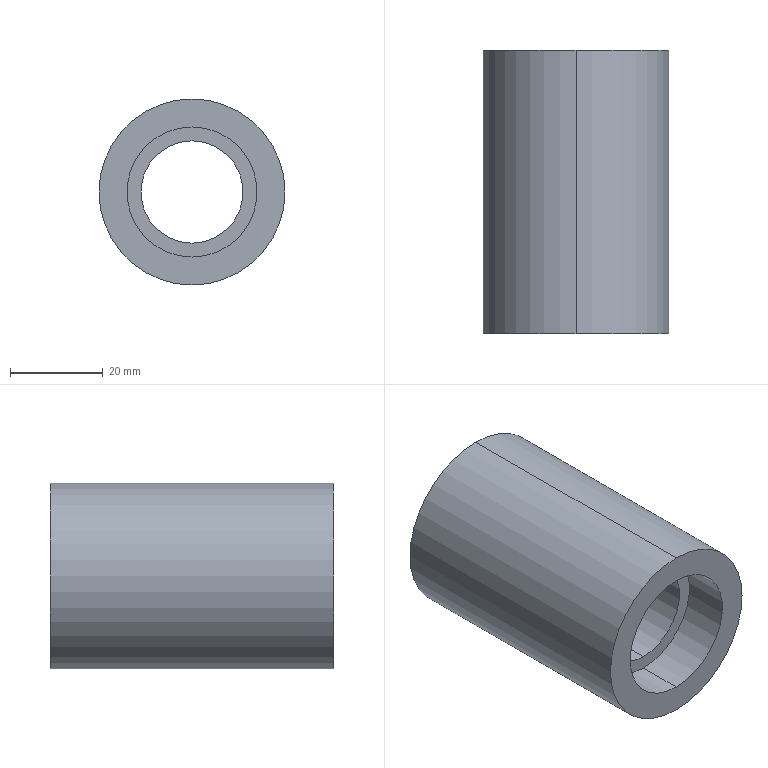Part | STEP file | ND25021-01-JDKM-22-TL | 1 solid | 12 faces | box 40 x 61 x 40 mm | volume 48754 mm3 | cylinder 8 | plane 4 | commonest cylinder face diameters 28 x4 22 x2 40 x2
STEP:
#1=CARTESIAN_POINT('',(0.,0.,0.));
#2=DIRECTION('',(0.,0.,1.));
#3=DIRECTION('',(1.,0.,0.));
#4=AXIS2_PLACEMENT_3D('',#1,#2,#3);
#5=CARTESIAN_POINT('',(0.,-20.5,-14.));
#6=VERTEX_POINT('',#5);
#7=CARTESIAN_POINT('',(0.,-30.5,-14.));
#8=VERTEX_POINT('',#7);
#9=CARTESIAN_POINT('',(0.,-20.5,-14.));
#10=DIRECTION('',(0.,-1.,0.));
#11=VECTOR('',#10,1.);
#12=LINE('',#9,#11);
#13=CARTESIAN_POINT('',(0.,-20.5,0.));
#14=DIRECTION('',(0.,-1.,0.));
#15=DIRECTION('',(0.,0.,-1.));
#16=AXIS2_PLACEMENT_3D('',#13,#14,#15);
#17=CYLINDRICAL_SURFACE('',#16,14.);
#18=CARTESIAN_POINT('',(6.283,0.));
#19=DIRECTION('',(0.,1.));
#20=VECTOR('',#19,1.);
#21=LINE('',#18,#20);
#22=(GEOMETRIC_REPRESENTATION_CONTEXT(2)PARAMETRIC_REPRESENTATION_CONTEXT()REPRESENTATION_CONTEXT('',''));
#23=DEFINITIONAL_REPRESENTATION('',(#21),#22);
#24=PCURVE('',#17,#23);
#25=CARTESIAN_POINT('',(0.,-20.5,0.));
#26=DIRECTION('',(0.,-1.,0.));
#27=DIRECTION('',(0.,0.,-1.));
#28=AXIS2_PLACEMENT_3D('',#25,#26,#27);
#29=CYLINDRICAL_SURFACE('',#28,14.);
#30=CARTESIAN_POINT('',(0.,0.));
#31=DIRECTION('',(0.,1.));
#32=VECTOR('',#31,1.);
#33=LINE('',#30,#32);
#34=(GEOMETRIC_REPRESENTATION_CONTEXT(2)PARAMETRIC_REPRESENTATION_CONTEXT()REPRESENTATION_CONTEXT('',''));
#35=DEFINITIONAL_REPRESENTATION('',(#33),#34);
#36=PCURVE('',#29,#35);
#37=SURFACE_CURVE('',#12,(#24,#36),.PCURVE_S1.);
#38=EDGE_CURVE('',#6,#8,#37,.T.);
#39=ORIENTED_EDGE('',*,*,#38,.T.);
#40=CARTESIAN_POINT('',(0.,-30.5,14.));
#41=VERTEX_POINT('',#40);
#42=CARTESIAN_POINT('',(0.,-30.5,0.));
#43=DIRECTION('',(0.,-1.,0.));
#44=DIRECTION('',(0.,0.,-1.));
#45=AXIS2_PLACEMENT_3D('',#42,#43,#44);
#46=CIRCLE('',#45,14.);
#47=CARTESIAN_POINT('',(0.,10.));
#48=DIRECTION('',(1.,0.));
#49=VECTOR('',#48,1.);
#50=LINE('',#47,#49);
#51=(GEOMETRIC_REPRESENTATION_CONTEXT(2)PARAMETRIC_REPRESENTATION_CONTEXT()REPRESENTATION_CONTEXT('',''));
#52=DEFINITIONAL_REPRESENTATION('',(#50),#51);
#53=PCURVE('',#17,#52);
#54=CARTESIAN_POINT('',(0.,-30.5,0.));
#55=DIRECTION('',(0.,1.,0.));
#56=DIRECTION('',(0.,0.,1.));
#57=AXIS2_PLACEMENT_3D('',#54,#55,#56);
#58=PLANE('',#57);
#59=CARTESIAN_POINT('',(-14.,0.));
#60=CARTESIAN_POINT('',(-14.,24.249));
#61=CARTESIAN_POINT('',(7.,12.124));
#62=CARTESIAN_POINT('',(28.,0.));
#63=CARTESIAN_POINT('',(7.,-12.124));
#64=CARTESIAN_POINT('',(-14.,-24.249));
#65=CARTESIAN_POINT('',(-14.,0.));
#66=(BOUNDED_CURVE()B_SPLINE_CURVE(2,(#59,#60,#61,#62,#63,#64,#65),.UNSPECIFIED.,.T.,.F.)B_SPLINE_CURVE_WITH_KNOTS((1,2,2,2,2,1),(-2.094,0.,2.094,4.189,6.283,8.378),.UNSPECIFIED.)CURVE()GEOMETRIC_REPRESENTATION_ITEM()RATIONAL_B_SPLINE_CURVE((1.,0.5,1.,0.5,1.,0.5,1.))REPRESENTATION_ITEM(''));
#67=(GEOMETRIC_REPRESENTATION_CONTEXT(2)PARAMETRIC_REPRESENTATION_CONTEXT()REPRESENTATION_CONTEXT('',''));
#68=DEFINITIONAL_REPRESENTATION('',(#66),#67);
#69=PCURVE('',#58,#68);
#70=SURFACE_CURVE('',#46,(#53,#69),.PCURVE_S1.);
#71=EDGE_CURVE('',#41,#8,#70,.T.);
#72=ORIENTED_EDGE('',*,*,#71,.F.);
#73=CARTESIAN_POINT('',(0.,-20.5,14.));
#74=VERTEX_POINT('',#73);
#75=CARTESIAN_POINT('',(0.,-20.5,14.));
#76=DIRECTION('',(0.,-1.,0.));
#77=VECTOR('',#76,1.);
#78=LINE('',#75,#77);
#79=CARTESIAN_POINT('',(3.142,0.));
#80=DIRECTION('',(0.,1.));
#81=VECTOR('',#80,1.);
#82=LINE('',#79,#81);
#83=(GEOMETRIC_REPRESENTATION_CONTEXT(2)PARAMETRIC_REPRESENTATION_CONTEXT()REPRESENTATION_CONTEXT('',''));
#84=DEFINITIONAL_REPRESENTATION('',(#82),#83);
#85=PCURVE('',#17,#84);
#86=CARTESIAN_POINT('',(3.142,0.));
#87=DIRECTION('',(0.,1.));
#88=VECTOR('',#87,1.);
#89=LINE('',#86,#88);
#90=(GEOMETRIC_REPRESENTATION_CONTEXT(2)PARAMETRIC_REPRESENTATION_CONTEXT()REPRESENTATION_CONTEXT('',''));
#91=DEFINITIONAL_REPRESENTATION('',(#89),#90);
#92=PCURVE('',#29,#91);
#93=SURFACE_CURVE('',#78,(#85,#92),.PCURVE_S1.);
#94=EDGE_CURVE('',#74,#41,#93,.T.);
#95=ORIENTED_EDGE('',*,*,#94,.F.);
#96=CARTESIAN_POINT('',(0.,-20.5,0.));
#97=DIRECTION('',(0.,-1.,0.));
#98=DIRECTION('',(0.,0.,-1.));
#99=AXIS2_PLACEMENT_3D('',#96,#97,#98);
#100=CIRCLE('',#99,14.);
#101=CARTESIAN_POINT('',(0.,0.));
#102=DIRECTION('',(1.,0.));
#103=VECTOR('',#102,1.);
#104=LINE('',#101,#103);
#105=(GEOMETRIC_REPRESENTATION_CONTEXT(2)PARAMETRIC_REPRESENTATION_CONTEXT()REPRESENTATION_CONTEXT('',''));
#106=DEFINITIONAL_REPRESENTATION('',(#104),#105);
#107=PCURVE('',#17,#106);
#108=CARTESIAN_POINT('',(0.,-20.5,0.));
#109=DIRECTION('',(0.,-1.,0.));
#110=DIRECTION('',(0.,0.,-1.));
#111=AXIS2_PLACEMENT_3D('',#108,#109,#110);
#112=PLANE('',#111);
#113=CARTESIAN_POINT('',(0.,0.));
#114=DIRECTION('',(1.,0.));
#115=AXIS2_PLACEMENT_2D('',#113,#114);
#116=CIRCLE('',#115,14.);
#117=(GEOMETRIC_REPRESENTATION_CONTEXT(2)PARAMETRIC_REPRESENTATION_CONTEXT()REPRESENTATION_CONTEXT('',''));
#118=DEFINITIONAL_REPRESENTATION('',(#116),#117);
#119=PCURVE('',#112,#118);
#120=SURFACE_CURVE('',#100,(#107,#119),.PCURVE_S1.);
#121=EDGE_CURVE('',#74,#6,#120,.T.);
#122=ORIENTED_EDGE('',*,*,#121,.T.);
#123=EDGE_LOOP('',(#39,#72,#95,#122));
#124=FACE_BOUND('',#123,.F.);
#125=ADVANCED_FACE('',(#124),#17,.F.);
#126=CARTESIAN_POINT('',(0.,20.5,14.));
#127=VERTEX_POINT('',#126);
#128=CARTESIAN_POINT('',(0.,30.5,14.));
#129=VERTEX_POINT('',#128);
#130=CARTESIAN_POINT('',(0.,20.5,14.));
#131=DIRECTION('',(0.,1.,0.));
#132=VECTOR('',#131,1.);
#133=LINE('',#130,#132);
#134=CARTESIAN_POINT('',(0.,20.5,0.));
#135=DIRECTION('',(0.,1.,0.));
#136=DIRECTION('',(0.,0.,1.));
#137=AXIS2_PLACEMENT_3D('',#134,#135,#136);
#138=CYLINDRICAL_SURFACE('',#137,14.);
#139=CARTESIAN_POINT('',(6.283,0.));
#140=DIRECTION('',(0.,1.));
#141=VECTOR('',#140,1.);
#142=LINE('',#139,#141);
#143=(GEOMETRIC_REPRESENTATION_CONTEXT(2)PARAMETRIC_REPRESENTATION_CONTEXT()REPRESENTATION_CONTEXT('',''));
#144=DEFINITIONAL_REPRESENTATION('',(#142),#143);
#145=PCURVE('',#138,#144);
#146=CARTESIAN_POINT('',(0.,20.5,0.));
#147=DIRECTION('',(0.,1.,0.));
#148=DIRECTION('',(0.,0.,1.));
#149=AXIS2_PLACEMENT_3D('',#146,#147,#148);
#150=CYLINDRICAL_SURFACE('',#149,14.);
#151=CARTESIAN_POINT('',(0.,0.));
#152=DIRECTION('',(0.,1.));
#153=VECTOR('',#152,1.);
#154=LINE('',#151,#153);
#155=(GEOMETRIC_REPRESENTATION_CONTEXT(2)PARAMETRIC_REPRESENTATION_CONTEXT()REPRESENTATION_CONTEXT('',''));
#156=DEFINITIONAL_REPRESENTATION('',(#154),#155);
#157=PCURVE('',#150,#156);
#158=SURFACE_CURVE('',#133,(#145,#157),.PCURVE_S1.);
#159=EDGE_CURVE('',#127,#129,#158,.T.);
#160=ORIENTED_EDGE('',*,*,#159,.T.);
#161=CARTESIAN_POINT('',(0.,30.5,-14.));
#162=VERTEX_POINT('',#161);
#163=CARTESIAN_POINT('',(0.,30.5,0.));
#164=DIRECTION('',(0.,1.,0.));
#165=DIRECTION('',(0.,0.,1.));
#166=AXIS2_PLACEMENT_3D('',#163,#164,#165);
#167=CIRCLE('',#166,14.);
#168=CARTESIAN_POINT('',(0.,10.));
#169=DIRECTION('',(1.,0.));
#170=VECTOR('',#169,1.);
#171=LINE('',#168,#170);
#172=(GEOMETRIC_REPRESENTATION_CONTEXT(2)PARAMETRIC_REPRESENTATION_CONTEXT()REPRESENTATION_CONTEXT('',''));
#173=DEFINITIONAL_REPRESENTATION('',(#171),#172);
#174=PCURVE('',#138,#173);
#175=CARTESIAN_POINT('',(0.,30.5,0.));
#176=DIRECTION('',(0.,1.,0.));
#177=DIRECTION('',(0.,0.,1.));
#178=AXIS2_PLACEMENT_3D('',#175,#176,#177);
#179=PLANE('',#178);
#180=CARTESIAN_POINT('',(0.,0.));
#181=DIRECTION('',(1.,0.));
#182=AXIS2_PLACEMENT_2D('',#180,#181);
#183=CIRCLE('',#182,14.);
#184=(GEOMETRIC_REPRESENTATION_CONTEXT(2)PARAMETRIC_REPRESENTATION_CONTEXT()REPRESENTATION_CONTEXT('',''));
#185=DEFINITIONAL_REPRESENTATION('',(#183),#184);
#186=PCURVE('',#179,#185);
#187=SURFACE_CURVE('',#167,(#174,#186),.PCURVE_S1.);
#188=EDGE_CURVE('',#162,#129,#187,.T.);
#189=ORIENTED_EDGE('',*,*,#188,.F.);
#190=CARTESIAN_POINT('',(0.,20.5,-14.));
#191=VERTEX_POINT('',#190);
#192=CARTESIAN_POINT('',(0.,20.5,-14.));
#193=DIRECTION('',(0.,1.,0.));
#194=VECTOR('',#193,1.);
#195=LINE('',#192,#194);
#196=CARTESIAN_POINT('',(3.142,0.));
#197=DIRECTION('',(0.,1.));
#198=VECTOR('',#197,1.);
#199=LINE('',#196,#198);
#200=(GEOMETRIC_REPRESENTATION_CONTEXT(2)PARAMETRIC_REPRESENTATION_CONTEXT()REPRESENTATION_CONTEXT('',''));
#201=DEFINITIONAL_REPRESENTATION('',(#199),#200);
#202=PCURVE('',#138,#201);
#203=CARTESIAN_POINT('',(3.142,0.));
#204=DIRECTION('',(0.,1.));
#205=VECTOR('',#204,1.);
#206=LINE('',#203,#205);
#207=(GEOMETRIC_REPRESENTATION_CONTEXT(2)PARAMETRIC_REPRESENTATION_CONTEXT()REPRESENTATION_CONTEXT('',''));
#208=DEFINITIONAL_REPRESENTATION('',(#206),#207);
#209=PCURVE('',#150,#208);
#210=SURFACE_CURVE('',#195,(#202,#209),.PCURVE_S1.);
#211=EDGE_CURVE('',#191,#162,#210,.T.);
#212=ORIENTED_EDGE('',*,*,#211,.F.);
#213=CARTESIAN_POINT('',(0.,20.5,0.));
#214=DIRECTION('',(0.,1.,0.));
#215=DIRECTION('',(0.,0.,1.));
#216=AXIS2_PLACEMENT_3D('',#213,#214,#215);
#217=CIRCLE('',#216,14.);
#218=CARTESIAN_POINT('',(0.,0.));
#219=DIRECTION('',(1.,0.));
#220=VECTOR('',#219,1.);
#221=LINE('',#218,#220);
#222=(GEOMETRIC_REPRESENTATION_CONTEXT(2)PARAMETRIC_REPRESENTATION_CONTEXT()REPRESENTATION_CONTEXT('',''));
#223=DEFINITIONAL_REPRESENTATION('',(#221),#222);
#224=PCURVE('',#138,#223);
#225=CARTESIAN_POINT('',(0.,20.5,0.));
#226=DIRECTION('',(0.,1.,0.));
#227=DIRECTION('',(0.,0.,1.));
#228=AXIS2_PLACEMENT_3D('',#225,#226,#227);
#229=PLANE('',#228);
#230=CARTESIAN_POINT('',(0.,0.));
#231=DIRECTION('',(1.,0.));
#232=AXIS2_PLACEMENT_2D('',#230,#231);
#233=CIRCLE('',#232,14.);
#234=(GEOMETRIC_REPRESENTATION_CONTEXT(2)PARAMETRIC_REPRESENTATION_CONTEXT()REPRESENTATION_CONTEXT('',''));
#235=DEFINITIONAL_REPRESENTATION('',(#233),#234);
#236=PCURVE('',#229,#235);
#237=SURFACE_CURVE('',#217,(#224,#236),.PCURVE_S1.);
#238=EDGE_CURVE('',#191,#127,#237,.T.);
#239=ORIENTED_EDGE('',*,*,#238,.T.);
#240=EDGE_LOOP('',(#160,#189,#212,#239));
#241=FACE_BOUND('',#240,.F.);
#242=ADVANCED_FACE('',(#241),#138,.F.);
#243=CARTESIAN_POINT('',(0.,30.5,20.));
#244=VERTEX_POINT('',#243);
#245=CARTESIAN_POINT('',(0.,30.5,-20.));
#246=VERTEX_POINT('',#245);
#247=CARTESIAN_POINT('',(0.,30.5,0.));
#248=DIRECTION('',(0.,1.,0.));
#249=DIRECTION('',(0.,0.,1.));
#250=AXIS2_PLACEMENT_3D('',#247,#248,#249);
#251=CIRCLE('',#250,20.);
#252=CARTESIAN_POINT('',(0.,30.5,0.));
#253=DIRECTION('',(0.,-1.,0.));
#254=DIRECTION('',(0.,0.,-1.));
#255=AXIS2_PLACEMENT_3D('',#252,#253,#254);
#256=CYLINDRICAL_SURFACE('',#255,20.);
#257=CARTESIAN_POINT('',(3.142,0.));
#258=DIRECTION('',(-1.,0.));
#259=VECTOR('',#258,1.);
#260=LINE('',#257,#259);
#261=(GEOMETRIC_REPRESENTATION_CONTEXT(2)PARAMETRIC_REPRESENTATION_CONTEXT()REPRESENTATION_CONTEXT('',''));
#262=DEFINITIONAL_REPRESENTATION('',(#260),#261);
#263=PCURVE('',#256,#262);
#264=CARTESIAN_POINT('',(0.,0.));
#265=DIRECTION('',(1.,0.));
#266=AXIS2_PLACEMENT_2D('',#264,#265);
#267=CIRCLE('',#266,20.);
#268=(GEOMETRIC_REPRESENTATION_CONTEXT(2)PARAMETRIC_REPRESENTATION_CONTEXT()REPRESENTATION_CONTEXT('',''));
#269=DEFINITIONAL_REPRESENTATION('',(#267),#268);
#270=PCURVE('',#179,#269);
#271=SURFACE_CURVE('',#251,(#263,#270),.PCURVE_S1.);
#272=EDGE_CURVE('',#244,#246,#271,.T.);
#273=ORIENTED_EDGE('',*,*,#272,.F.);
#274=CARTESIAN_POINT('',(0.,-30.5,20.));
#275=VERTEX_POINT('',#274);
#276=CARTESIAN_POINT('',(0.,30.5,20.));
#277=DIRECTION('',(0.,-1.,0.));
#278=VECTOR('',#277,1.);
#279=LINE('',#276,#278);
#280=CARTESIAN_POINT('',(3.142,0.));
#281=DIRECTION('',(0.,1.));
#282=VECTOR('',#281,1.);
#283=LINE('',#280,#282);
#284=(GEOMETRIC_REPRESENTATION_CONTEXT(2)PARAMETRIC_REPRESENTATION_CONTEXT()REPRESENTATION_CONTEXT('',''));
#285=DEFINITIONAL_REPRESENTATION('',(#283),#284);
#286=PCURVE('',#256,#285);
#287=CARTESIAN_POINT('',(0.,30.5,0.));
#288=DIRECTION('',(0.,-1.,0.));
#289=DIRECTION('',(0.,0.,-1.));
#290=AXIS2_PLACEMENT_3D('',#287,#288,#289);
#291=CYLINDRICAL_SURFACE('',#290,20.);
#292=CARTESIAN_POINT('',(3.142,0.));
#293=DIRECTION('',(0.,1.));
#294=VECTOR('',#293,1.);
#295=LINE('',#292,#294);
#296=(GEOMETRIC_REPRESENTATION_CONTEXT(2)PARAMETRIC_REPRESENTATION_CONTEXT()REPRESENTATION_CONTEXT('',''));
#297=DEFINITIONAL_REPRESENTATION('',(#295),#296);
#298=PCURVE('',#291,#297);
#299=SURFACE_CURVE('',#279,(#286,#298),.PCURVE_S1.);
#300=EDGE_CURVE('',#244,#275,#299,.T.);
#301=ORIENTED_EDGE('',*,*,#300,.T.);
#302=CARTESIAN_POINT('',(0.,-30.5,-20.));
#303=VERTEX_POINT('',#302);
#304=CARTESIAN_POINT('',(0.,-30.5,0.));
#305=DIRECTION('',(0.,1.,0.));
#306=DIRECTION('',(0.,0.,1.));
#307=AXIS2_PLACEMENT_3D('',#304,#305,#306);
#308=CIRCLE('',#307,20.);
#309=CARTESIAN_POINT('',(3.142,61.));
#310=DIRECTION('',(-1.,0.));
#311=VECTOR('',#310,1.);
#312=LINE('',#309,#311);
#313=(GEOMETRIC_REPRESENTATION_CONTEXT(2)PARAMETRIC_REPRESENTATION_CONTEXT()REPRESENTATION_CONTEXT('',''));
#314=DEFINITIONAL_REPRESENTATION('',(#312),#313);
#315=PCURVE('',#256,#314);
#316=CARTESIAN_POINT('',(0.,0.));
#317=DIRECTION('',(1.,0.));
#318=AXIS2_PLACEMENT_2D('',#316,#317);
#319=CIRCLE('',#318,20.);
#320=(GEOMETRIC_REPRESENTATION_CONTEXT(2)PARAMETRIC_REPRESENTATION_CONTEXT()REPRESENTATION_CONTEXT('',''));
#321=DEFINITIONAL_REPRESENTATION('',(#319),#320);
#322=PCURVE('',#58,#321);
#323=SURFACE_CURVE('',#308,(#315,#322),.PCURVE_S1.);
#324=EDGE_CURVE('',#275,#303,#323,.T.);
#325=ORIENTED_EDGE('',*,*,#324,.T.);
#326=CARTESIAN_POINT('',(0.,30.5,-20.));
#327=DIRECTION('',(0.,-1.,0.));
#328=VECTOR('',#327,1.);
#329=LINE('',#326,#328);
#330=CARTESIAN_POINT('',(0.,0.));
#331=DIRECTION('',(0.,1.));
#332=VECTOR('',#331,1.);
#333=LINE('',#330,#332);
#334=(GEOMETRIC_REPRESENTATION_CONTEXT(2)PARAMETRIC_REPRESENTATION_CONTEXT()REPRESENTATION_CONTEXT('',''));
#335=DEFINITIONAL_REPRESENTATION('',(#333),#334);
#336=PCURVE('',#256,#335);
#337=CARTESIAN_POINT('',(6.283,0.));
#338=DIRECTION('',(0.,1.));
#339=VECTOR('',#338,1.);
#340=LINE('',#337,#339);
#341=(GEOMETRIC_REPRESENTATION_CONTEXT(2)PARAMETRIC_REPRESENTATION_CONTEXT()REPRESENTATION_CONTEXT('',''));
#342=DEFINITIONAL_REPRESENTATION('',(#340),#341);
#343=PCURVE('',#291,#342);
#344=SURFACE_CURVE('',#329,(#336,#343),.PCURVE_S1.);
#345=EDGE_CURVE('',#246,#303,#344,.T.);
#346=ORIENTED_EDGE('',*,*,#345,.F.);
#347=EDGE_LOOP('',(#273,#301,#325,#346));
#348=FACE_BOUND('',#347,.T.);
#349=ADVANCED_FACE('',(#348),#256,.T.);
#350=CARTESIAN_POINT('',(0.,-20.5,11.));
#351=VERTEX_POINT('',#350);
#352=CARTESIAN_POINT('',(0.,20.5,11.));
#353=VERTEX_POINT('',#352);
#354=CARTESIAN_POINT('',(0.,-30.5,11.));
#355=DIRECTION('',(0.,1.,0.));
#356=VECTOR('',#355,1.);
#357=LINE('',#354,#356);
#358=CARTESIAN_POINT('',(0.,-30.5,0.));
#359=DIRECTION('',(0.,1.,0.));
#360=DIRECTION('',(0.,0.,1.));
#361=AXIS2_PLACEMENT_3D('',#358,#359,#360);
#362=CYLINDRICAL_SURFACE('',#361,11.);
#363=CARTESIAN_POINT('',(6.283,0.));
#364=DIRECTION('',(0.,1.));
#365=VECTOR('',#364,1.);
#366=LINE('',#363,#365);
#367=(GEOMETRIC_REPRESENTATION_CONTEXT(2)PARAMETRIC_REPRESENTATION_CONTEXT()REPRESENTATION_CONTEXT('',''));
#368=DEFINITIONAL_REPRESENTATION('',(#366),#367);
#369=PCURVE('',#362,#368);
#370=CARTESIAN_POINT('',(0.,-30.5,0.));
#371=DIRECTION('',(0.,1.,0.));
#372=DIRECTION('',(0.,0.,1.));
#373=AXIS2_PLACEMENT_3D('',#370,#371,#372);
#374=CYLINDRICAL_SURFACE('',#373,11.);
#375=CARTESIAN_POINT('',(0.,0.));
#376=DIRECTION('',(0.,1.));
#377=VECTOR('',#376,1.);
#378=LINE('',#375,#377);
#379=(GEOMETRIC_REPRESENTATION_CONTEXT(2)PARAMETRIC_REPRESENTATION_CONTEXT()REPRESENTATION_CONTEXT('',''));
#380=DEFINITIONAL_REPRESENTATION('',(#378),#379);
#381=PCURVE('',#374,#380);
#382=SURFACE_CURVE('',#357,(#369,#381),.PCURVE_S1.);
#383=EDGE_CURVE('',#351,#353,#382,.T.);
#384=ORIENTED_EDGE('',*,*,#383,.T.);
#385=CARTESIAN_POINT('',(0.,20.5,-11.));
#386=VERTEX_POINT('',#385);
#387=CARTESIAN_POINT('',(0.,20.5,0.));
#388=DIRECTION('',(0.,-1.,0.));
#389=DIRECTION('',(0.,0.,1.));
#390=AXIS2_PLACEMENT_3D('',#387,#388,#389);
#391=CIRCLE('',#390,11.);
#392=CARTESIAN_POINT('',(6.283,51.));
#393=DIRECTION('',(-1.,0.));
#394=VECTOR('',#393,1.);
#395=LINE('',#392,#394);
#396=(GEOMETRIC_REPRESENTATION_CONTEXT(2)PARAMETRIC_REPRESENTATION_CONTEXT()REPRESENTATION_CONTEXT('',''));
#397=DEFINITIONAL_REPRESENTATION('',(#395),#396);
#398=PCURVE('',#362,#397);
#399=CARTESIAN_POINT('',(11.,0.));
#400=CARTESIAN_POINT('',(11.,-19.053));
#401=CARTESIAN_POINT('',(-5.5,-9.526));
#402=CARTESIAN_POINT('',(-22.,0.));
#403=CARTESIAN_POINT('',(-5.5,9.526));
#404=CARTESIAN_POINT('',(11.,19.053));
#405=CARTESIAN_POINT('',(11.,0.));
#406=(BOUNDED_CURVE()B_SPLINE_CURVE(2,(#399,#400,#401,#402,#403,#404,#405),.UNSPECIFIED.,.T.,.F.)B_SPLINE_CURVE_WITH_KNOTS((1,2,2,2,2,1),(-2.094,0.,2.094,4.189,6.283,8.378),.UNSPECIFIED.)CURVE()GEOMETRIC_REPRESENTATION_ITEM()RATIONAL_B_SPLINE_CURVE((1.,0.5,1.,0.5,1.,0.5,1.))REPRESENTATION_ITEM(''));
#407=(GEOMETRIC_REPRESENTATION_CONTEXT(2)PARAMETRIC_REPRESENTATION_CONTEXT()REPRESENTATION_CONTEXT('',''));
#408=DEFINITIONAL_REPRESENTATION('',(#406),#407);
#409=PCURVE('',#229,#408);
#410=SURFACE_CURVE('',#391,(#398,#409),.PCURVE_S1.);
#411=EDGE_CURVE('',#353,#386,#410,.T.);
#412=ORIENTED_EDGE('',*,*,#411,.T.);
#413=CARTESIAN_POINT('',(0.,-20.5,-11.));
#414=VERTEX_POINT('',#413);
#415=CARTESIAN_POINT('',(0.,-30.5,-11.));
#416=DIRECTION('',(0.,1.,0.));
#417=VECTOR('',#416,1.);
#418=LINE('',#415,#417);
#419=CARTESIAN_POINT('',(3.142,0.));
#420=DIRECTION('',(0.,1.));
#421=VECTOR('',#420,1.);
#422=LINE('',#419,#421);
#423=(GEOMETRIC_REPRESENTATION_CONTEXT(2)PARAMETRIC_REPRESENTATION_CONTEXT()REPRESENTATION_CONTEXT('',''));
#424=DEFINITIONAL_REPRESENTATION('',(#422),#423);
#425=PCURVE('',#362,#424);
#426=CARTESIAN_POINT('',(3.142,0.));
#427=DIRECTION('',(0.,1.));
#428=VECTOR('',#427,1.);
#429=LINE('',#426,#428);
#430=(GEOMETRIC_REPRESENTATION_CONTEXT(2)PARAMETRIC_REPRESENTATION_CONTEXT()REPRESENTATION_CONTEXT('',''));
#431=DEFINITIONAL_REPRESENTATION('',(#429),#430);
#432=PCURVE('',#374,#431);
#433=SURFACE_CURVE('',#418,(#425,#432),.PCURVE_S1.);
#434=EDGE_CURVE('',#414,#386,#433,.T.);
#435=ORIENTED_EDGE('',*,*,#434,.F.);
#436=CARTESIAN_POINT('',(0.,-20.5,0.));
#437=DIRECTION('',(0.,1.,0.));
#438=DIRECTION('',(0.,0.,-1.));
#439=AXIS2_PLACEMENT_3D('',#436,#437,#438);
#440=CIRCLE('',#439,11.);
#441=CARTESIAN_POINT('',(3.142,10.));
#442=DIRECTION('',(1.,0.));
#443=VECTOR('',#442,1.);
#444=LINE('',#441,#443);
#445=(GEOMETRIC_REPRESENTATION_CONTEXT(2)PARAMETRIC_REPRESENTATION_CONTEXT()REPRESENTATION_CONTEXT('',''));
#446=DEFINITIONAL_REPRESENTATION('',(#444),#445);
#447=PCURVE('',#362,#446);
#448=CARTESIAN_POINT('',(11.,0.));
#449=CARTESIAN_POINT('',(11.,-19.053));
#450=CARTESIAN_POINT('',(-5.5,-9.526));
#451=CARTESIAN_POINT('',(-22.,0.));
#452=CARTESIAN_POINT('',(-5.5,9.526));
#453=CARTESIAN_POINT('',(11.,19.053));
#454=CARTESIAN_POINT('',(11.,0.));
#455=(BOUNDED_CURVE()B_SPLINE_CURVE(2,(#448,#449,#450,#451,#452,#453,#454),.UNSPECIFIED.,.T.,.F.)B_SPLINE_CURVE_WITH_KNOTS((1,2,2,2,2,1),(-2.094,0.,2.094,4.189,6.283,8.378),.UNSPECIFIED.)CURVE()GEOMETRIC_REPRESENTATION_ITEM()RATIONAL_B_SPLINE_CURVE((1.,0.5,1.,0.5,1.,0.5,1.))REPRESENTATION_ITEM(''));
#456=(GEOMETRIC_REPRESENTATION_CONTEXT(2)PARAMETRIC_REPRESENTATION_CONTEXT()REPRESENTATION_CONTEXT('',''));
#457=DEFINITIONAL_REPRESENTATION('',(#455),#456);
#458=PCURVE('',#112,#457);
#459=SURFACE_CURVE('',#440,(#447,#458),.PCURVE_S1.);
#460=EDGE_CURVE('',#414,#351,#459,.T.);
#461=ORIENTED_EDGE('',*,*,#460,.T.);
#462=EDGE_LOOP('',(#384,#412,#435,#461));
#463=FACE_BOUND('',#462,.F.);
#464=ADVANCED_FACE('',(#463),#362,.F.);
#465=CARTESIAN_POINT('',(0.,20.5,0.));
#466=DIRECTION('',(0.,-1.,0.));
#467=DIRECTION('',(0.,0.,1.));
#468=AXIS2_PLACEMENT_3D('',#465,#466,#467);
#469=CIRCLE('',#468,11.);
#470=CARTESIAN_POINT('',(6.283,51.));
#471=DIRECTION('',(-1.,0.));
#472=VECTOR('',#471,1.);
#473=LINE('',#470,#472);
#474=(GEOMETRIC_REPRESENTATION_CONTEXT(2)PARAMETRIC_REPRESENTATION_CONTEXT()REPRESENTATION_CONTEXT('',''));
#475=DEFINITIONAL_REPRESENTATION('',(#473),#474);
#476=PCURVE('',#374,#475);
#477=CARTESIAN_POINT('',(11.,0.));
#478=CARTESIAN_POINT('',(11.,-19.053));
#479=CARTESIAN_POINT('',(-5.5,-9.526));
#480=CARTESIAN_POINT('',(-22.,0.));
#481=CARTESIAN_POINT('',(-5.5,9.526));
#482=CARTESIAN_POINT('',(11.,19.053));
#483=CARTESIAN_POINT('',(11.,0.));
#484=(BOUNDED_CURVE()B_SPLINE_CURVE(2,(#477,#478,#479,#480,#481,#482,#483),.UNSPECIFIED.,.T.,.F.)B_SPLINE_CURVE_WITH_KNOTS((1,2,2,2,2,1),(-2.094,0.,2.094,4.189,6.283,8.378),.UNSPECIFIED.)CURVE()GEOMETRIC_REPRESENTATION_ITEM()RATIONAL_B_SPLINE_CURVE((1.,0.5,1.,0.5,1.,0.5,1.))REPRESENTATION_ITEM(''));
#485=(GEOMETRIC_REPRESENTATION_CONTEXT(2)PARAMETRIC_REPRESENTATION_CONTEXT()REPRESENTATION_CONTEXT('',''));
#486=DEFINITIONAL_REPRESENTATION('',(#484),#485);
#487=PCURVE('',#229,#486);
#488=SURFACE_CURVE('',#469,(#476,#487),.PCURVE_S1.);
#489=EDGE_CURVE('',#386,#353,#488,.T.);
#490=ORIENTED_EDGE('',*,*,#489,.T.);
#491=ORIENTED_EDGE('',*,*,#383,.F.);
#492=CARTESIAN_POINT('',(0.,-20.5,0.));
#493=DIRECTION('',(0.,1.,0.));
#494=DIRECTION('',(0.,0.,-1.));
#495=AXIS2_PLACEMENT_3D('',#492,#493,#494);
#496=CIRCLE('',#495,11.);
#497=CARTESIAN_POINT('',(-3.142,10.));
#498=DIRECTION('',(1.,0.));
#499=VECTOR('',#498,1.);
#500=LINE('',#497,#499);
#501=(GEOMETRIC_REPRESENTATION_CONTEXT(2)PARAMETRIC_REPRESENTATION_CONTEXT()REPRESENTATION_CONTEXT('',''));
#502=DEFINITIONAL_REPRESENTATION('',(#500),#501);
#503=PCURVE('',#374,#502);
#504=CARTESIAN_POINT('',(11.,0.));
#505=CARTESIAN_POINT('',(11.,-19.053));
#506=CARTESIAN_POINT('',(-5.5,-9.526));
#507=CARTESIAN_POINT('',(-22.,0.));
#508=CARTESIAN_POINT('',(-5.5,9.526));
#509=CARTESIAN_POINT('',(11.,19.053));
#510=CARTESIAN_POINT('',(11.,0.));
#511=(BOUNDED_CURVE()B_SPLINE_CURVE(2,(#504,#505,#506,#507,#508,#509,#510),.UNSPECIFIED.,.T.,.F.)B_SPLINE_CURVE_WITH_KNOTS((1,2,2,2,2,1),(-2.094,0.,2.094,4.189,6.283,8.378),.UNSPECIFIED.)CURVE()GEOMETRIC_REPRESENTATION_ITEM()RATIONAL_B_SPLINE_CURVE((1.,0.5,1.,0.5,1.,0.5,1.))REPRESENTATION_ITEM(''));
#512=(GEOMETRIC_REPRESENTATION_CONTEXT(2)PARAMETRIC_REPRESENTATION_CONTEXT()REPRESENTATION_CONTEXT('',''));
#513=DEFINITIONAL_REPRESENTATION('',(#511),#512);
#514=PCURVE('',#112,#513);
#515=SURFACE_CURVE('',#496,(#503,#514),.PCURVE_S1.);
#516=EDGE_CURVE('',#351,#414,#515,.T.);
#517=ORIENTED_EDGE('',*,*,#516,.T.);
#518=ORIENTED_EDGE('',*,*,#434,.T.);
#519=EDGE_LOOP('',(#490,#491,#517,#518));
#520=FACE_BOUND('',#519,.F.);
#521=ADVANCED_FACE('',(#520),#374,.F.);
#522=ORIENTED_EDGE('',*,*,#300,.F.);
#523=CARTESIAN_POINT('',(0.,30.5,0.));
#524=DIRECTION('',(0.,1.,0.));
#525=DIRECTION('',(0.,0.,1.));
#526=AXIS2_PLACEMENT_3D('',#523,#524,#525);
#527=CIRCLE('',#526,20.);
#528=CARTESIAN_POINT('',(9.425,0.));
#529=DIRECTION('',(-1.,0.));
#530=VECTOR('',#529,1.);
#531=LINE('',#528,#530);
#532=(GEOMETRIC_REPRESENTATION_CONTEXT(2)PARAMETRIC_REPRESENTATION_CONTEXT()REPRESENTATION_CONTEXT('',''));
#533=DEFINITIONAL_REPRESENTATION('',(#531),#532);
#534=PCURVE('',#291,#533);
#535=CARTESIAN_POINT('',(0.,0.));
#536=DIRECTION('',(1.,0.));
#537=AXIS2_PLACEMENT_2D('',#535,#536);
#538=CIRCLE('',#537,20.);
#539=(GEOMETRIC_REPRESENTATION_CONTEXT(2)PARAMETRIC_REPRESENTATION_CONTEXT()REPRESENTATION_CONTEXT('',''));
#540=DEFINITIONAL_REPRESENTATION('',(#538),#539);
#541=PCURVE('',#179,#540);
#542=SURFACE_CURVE('',#527,(#534,#541),.PCURVE_S1.);
#543=EDGE_CURVE('',#246,#244,#542,.T.);
#544=ORIENTED_EDGE('',*,*,#543,.F.);
#545=ORIENTED_EDGE('',*,*,#345,.T.);
#546=CARTESIAN_POINT('',(0.,-30.5,0.));
#547=DIRECTION('',(0.,1.,0.));
#548=DIRECTION('',(0.,0.,1.));
#549=AXIS2_PLACEMENT_3D('',#546,#547,#548);
#550=CIRCLE('',#549,20.);
#551=CARTESIAN_POINT('',(9.425,61.));
#552=DIRECTION('',(-1.,0.));
#553=VECTOR('',#552,1.);
#554=LINE('',#551,#553);
#555=(GEOMETRIC_REPRESENTATION_CONTEXT(2)PARAMETRIC_REPRESENTATION_CONTEXT()REPRESENTATION_CONTEXT('',''));
#556=DEFINITIONAL_REPRESENTATION('',(#554),#555);
#557=PCURVE('',#291,#556);
#558=CARTESIAN_POINT('',(0.,0.));
#559=DIRECTION('',(1.,0.));
#560=AXIS2_PLACEMENT_2D('',#558,#559);
#561=CIRCLE('',#560,20.);
#562=(GEOMETRIC_REPRESENTATION_CONTEXT(2)PARAMETRIC_REPRESENTATION_CONTEXT()REPRESENTATION_CONTEXT('',''));
#563=DEFINITIONAL_REPRESENTATION('',(#561),#562);
#564=PCURVE('',#58,#563);
#565=SURFACE_CURVE('',#550,(#557,#564),.PCURVE_S1.);
#566=EDGE_CURVE('',#303,#275,#565,.T.);
#567=ORIENTED_EDGE('',*,*,#566,.T.);
#568=EDGE_LOOP('',(#522,#544,#545,#567));
#569=FACE_BOUND('',#568,.T.);
#570=ADVANCED_FACE('',(#569),#291,.T.);
#571=CARTESIAN_POINT('',(0.,30.5,0.));
#572=DIRECTION('',(0.,1.,0.));
#573=DIRECTION('',(0.,0.,1.));
#574=AXIS2_PLACEMENT_3D('',#571,#572,#573);
#575=CIRCLE('',#574,14.);
#576=CARTESIAN_POINT('',(0.,0.));
#577=DIRECTION('',(1.,0.));
#578=AXIS2_PLACEMENT_2D('',#576,#577);
#579=CIRCLE('',#578,14.);
#580=(GEOMETRIC_REPRESENTATION_CONTEXT(2)PARAMETRIC_REPRESENTATION_CONTEXT()REPRESENTATION_CONTEXT('',''));
#581=DEFINITIONAL_REPRESENTATION('',(#579),#580);
#582=PCURVE('',#179,#581);
#583=CARTESIAN_POINT('',(0.,10.));
#584=DIRECTION('',(1.,0.));
#585=VECTOR('',#584,1.);
#586=LINE('',#583,#585);
#587=(GEOMETRIC_REPRESENTATION_CONTEXT(2)PARAMETRIC_REPRESENTATION_CONTEXT()REPRESENTATION_CONTEXT('',''));
#588=DEFINITIONAL_REPRESENTATION('',(#586),#587);
#589=PCURVE('',#150,#588);
#590=SURFACE_CURVE('',#575,(#582,#589),.PCURVE_S1.);
#591=EDGE_CURVE('',#129,#162,#590,.T.);
#592=ORIENTED_EDGE('',*,*,#591,.F.);
#593=ORIENTED_EDGE('',*,*,#188,.F.);
#594=EDGE_LOOP('',(#592,#593));
#595=FACE_BOUND('',#594,.T.);
#596=ORIENTED_EDGE('',*,*,#543,.T.);
#597=ORIENTED_EDGE('',*,*,#272,.T.);
#598=EDGE_LOOP('',(#596,#597));
#599=FACE_BOUND('',#598,.T.);
#600=ADVANCED_FACE('',(#595,#599),#179,.T.);
#601=CARTESIAN_POINT('',(0.,-30.5,0.));
#602=DIRECTION('',(0.,-1.,0.));
#603=DIRECTION('',(0.,0.,-1.));
#604=AXIS2_PLACEMENT_3D('',#601,#602,#603);
#605=CIRCLE('',#604,14.);
#606=CARTESIAN_POINT('',(-14.,0.));
#607=CARTESIAN_POINT('',(-14.,24.249));
#608=CARTESIAN_POINT('',(7.,12.124));
#609=CARTESIAN_POINT('',(28.,0.));
#610=CARTESIAN_POINT('',(7.,-12.124));
#611=CARTESIAN_POINT('',(-14.,-24.249));
#612=CARTESIAN_POINT('',(-14.,0.));
#613=(BOUNDED_CURVE()B_SPLINE_CURVE(2,(#606,#607,#608,#609,#610,#611,#612),.UNSPECIFIED.,.T.,.F.)B_SPLINE_CURVE_WITH_KNOTS((1,2,2,2,2,1),(-2.094,0.,2.094,4.189,6.283,8.378),.UNSPECIFIED.)CURVE()GEOMETRIC_REPRESENTATION_ITEM()RATIONAL_B_SPLINE_CURVE((1.,0.5,1.,0.5,1.,0.5,1.))REPRESENTATION_ITEM(''));
#614=(GEOMETRIC_REPRESENTATION_CONTEXT(2)PARAMETRIC_REPRESENTATION_CONTEXT()REPRESENTATION_CONTEXT('',''));
#615=DEFINITIONAL_REPRESENTATION('',(#613),#614);
#616=PCURVE('',#58,#615);
#617=CARTESIAN_POINT('',(0.,10.));
#618=DIRECTION('',(1.,0.));
#619=VECTOR('',#618,1.);
#620=LINE('',#617,#619);
#621=(GEOMETRIC_REPRESENTATION_CONTEXT(2)PARAMETRIC_REPRESENTATION_CONTEXT()REPRESENTATION_CONTEXT('',''));
#622=DEFINITIONAL_REPRESENTATION('',(#620),#621);
#623=PCURVE('',#29,#622);
#624=SURFACE_CURVE('',#605,(#616,#623),.PCURVE_S1.);
#625=EDGE_CURVE('',#8,#41,#624,.T.);
#626=ORIENTED_EDGE('',*,*,#625,.F.);
#627=ORIENTED_EDGE('',*,*,#71,.F.);
#628=EDGE_LOOP('',(#626,#627));
#629=FACE_BOUND('',#628,.T.);
#630=ORIENTED_EDGE('',*,*,#566,.F.);
#631=ORIENTED_EDGE('',*,*,#324,.F.);
#632=EDGE_LOOP('',(#630,#631));
#633=FACE_BOUND('',#632,.T.);
#634=ADVANCED_FACE('',(#629,#633),#58,.F.);
#635=CARTESIAN_POINT('',(0.,20.5,0.));
#636=DIRECTION('',(0.,1.,0.));
#637=DIRECTION('',(0.,0.,1.));
#638=AXIS2_PLACEMENT_3D('',#635,#636,#637);
#639=CIRCLE('',#638,14.);
#640=CARTESIAN_POINT('',(0.,0.));
#641=DIRECTION('',(1.,0.));
#642=AXIS2_PLACEMENT_2D('',#640,#641);
#643=CIRCLE('',#642,14.);
#644=(GEOMETRIC_REPRESENTATION_CONTEXT(2)PARAMETRIC_REPRESENTATION_CONTEXT()REPRESENTATION_CONTEXT('',''));
#645=DEFINITIONAL_REPRESENTATION('',(#643),#644);
#646=PCURVE('',#229,#645);
#647=CARTESIAN_POINT('',(0.,0.));
#648=DIRECTION('',(1.,0.));
#649=VECTOR('',#648,1.);
#650=LINE('',#647,#649);
#651=(GEOMETRIC_REPRESENTATION_CONTEXT(2)PARAMETRIC_REPRESENTATION_CONTEXT()REPRESENTATION_CONTEXT('',''));
#652=DEFINITIONAL_REPRESENTATION('',(#650),#651);
#653=PCURVE('',#150,#652);
#654=SURFACE_CURVE('',#639,(#646,#653),.PCURVE_S1.);
#655=EDGE_CURVE('',#127,#191,#654,.T.);
#656=ORIENTED_EDGE('',*,*,#655,.T.);
#657=ORIENTED_EDGE('',*,*,#238,.T.);
#658=EDGE_LOOP('',(#656,#657));
#659=FACE_BOUND('',#658,.T.);
#660=ORIENTED_EDGE('',*,*,#411,.T.);
#661=ORIENTED_EDGE('',*,*,#489,.T.);
#662=EDGE_LOOP('',(#660,#661));
#663=FACE_BOUND('',#662,.T.);
#664=ADVANCED_FACE('',(#659,#663),#229,.T.);
#665=ORIENTED_EDGE('',*,*,#591,.F.);
#666=ORIENTED_EDGE('',*,*,#159,.F.);
#667=ORIENTED_EDGE('',*,*,#655,.T.);
#668=ORIENTED_EDGE('',*,*,#211,.T.);
#669=EDGE_LOOP('',(#665,#666,#667,#668));
#670=FACE_BOUND('',#669,.F.);
#671=ADVANCED_FACE('',(#670),#150,.F.);
#672=CARTESIAN_POINT('',(0.,-20.5,0.));
#673=DIRECTION('',(0.,-1.,0.));
#674=DIRECTION('',(0.,0.,-1.));
#675=AXIS2_PLACEMENT_3D('',#672,#673,#674);
#676=CIRCLE('',#675,14.);
#677=CARTESIAN_POINT('',(0.,0.));
#678=DIRECTION('',(1.,0.));
#679=AXIS2_PLACEMENT_2D('',#677,#678);
#680=CIRCLE('',#679,14.);
#681=(GEOMETRIC_REPRESENTATION_CONTEXT(2)PARAMETRIC_REPRESENTATION_CONTEXT()REPRESENTATION_CONTEXT('',''));
#682=DEFINITIONAL_REPRESENTATION('',(#680),#681);
#683=PCURVE('',#112,#682);
#684=CARTESIAN_POINT('',(0.,0.));
#685=DIRECTION('',(1.,0.));
#686=VECTOR('',#685,1.);
#687=LINE('',#684,#686);
#688=(GEOMETRIC_REPRESENTATION_CONTEXT(2)PARAMETRIC_REPRESENTATION_CONTEXT()REPRESENTATION_CONTEXT('',''));
#689=DEFINITIONAL_REPRESENTATION('',(#687),#688);
#690=PCURVE('',#29,#689);
#691=SURFACE_CURVE('',#676,(#683,#690),.PCURVE_S1.);
#692=EDGE_CURVE('',#6,#74,#691,.T.);
#693=ORIENTED_EDGE('',*,*,#692,.T.);
#694=ORIENTED_EDGE('',*,*,#121,.T.);
#695=EDGE_LOOP('',(#693,#694));
#696=FACE_BOUND('',#695,.T.);
#697=ORIENTED_EDGE('',*,*,#516,.T.);
#698=ORIENTED_EDGE('',*,*,#460,.T.);
#699=EDGE_LOOP('',(#697,#698));
#700=FACE_BOUND('',#699,.T.);
#701=ADVANCED_FACE('',(#696,#700),#112,.T.);
#702=ORIENTED_EDGE('',*,*,#625,.F.);
#703=ORIENTED_EDGE('',*,*,#38,.F.);
#704=ORIENTED_EDGE('',*,*,#692,.T.);
#705=ORIENTED_EDGE('',*,*,#94,.T.);
#706=EDGE_LOOP('',(#702,#703,#704,#705));
#707=FACE_BOUND('',#706,.F.);
#708=ADVANCED_FACE('',(#707),#29,.F.);
#709=CLOSED_SHELL('',(#125,#242,#349,#464,#521,#570,#600,#634,#664,#671,#701,#708));
#710=MANIFOLD_SOLID_BREP('',#709);
#711=(LENGTH_UNIT()NAMED_UNIT(*)SI_UNIT(.MILLI.,.METRE.));
#712=UNCERTAINTY_MEASURE_WITH_UNIT(LENGTH_MEASURE(0.0000001),#711,'','');
#713=(NAMED_UNIT(*)PLANE_ANGLE_UNIT()SI_UNIT($,.RADIAN.));
#714=(NAMED_UNIT(*)SI_UNIT($,.STERADIAN.)SOLID_ANGLE_UNIT());
#715=(GEOMETRIC_REPRESENTATION_CONTEXT(3)GLOBAL_UNCERTAINTY_ASSIGNED_CONTEXT((#712))GLOBAL_UNIT_ASSIGNED_CONTEXT((#711,#713,#714))REPRESENTATION_CONTEXT('',''));
#716=ADVANCED_BREP_SHAPE_REPRESENTATION('',(#4,#710),#715);